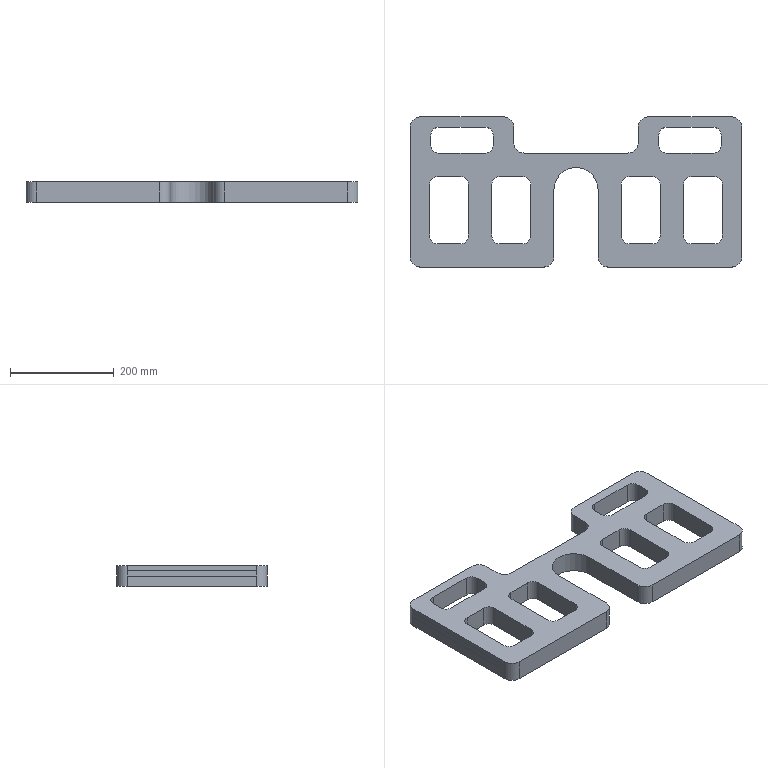Part | SolidWorks | features Fillet 2, Extrusion 1, ICE 1, MirrorPattern 1, PLine 1 | 1 solid | 76 faces | box 640 x 290 x 40 mm | volume 4114262 mm3 | plane 41 | cylinder 35 | commonest cylinder face diameters 30 x24 40 x10 85 x1